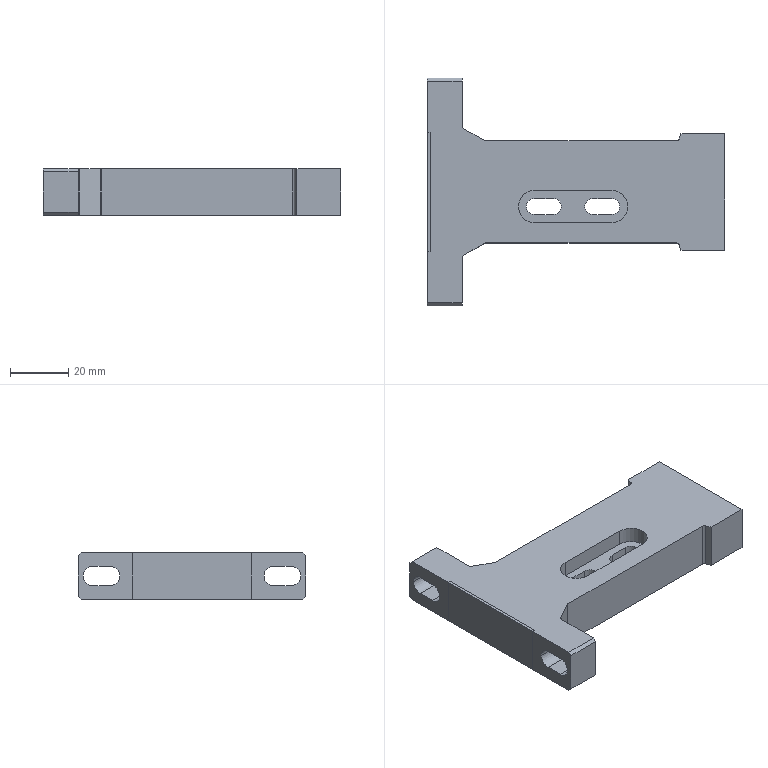NC program | NX | posted with a generic post | part box 102 x 78 x 16 mm
Lines 1 to 22 of 11044:
N10 G17 G21 G94 G90
(FLOOR_WALL , TOOL : D63)
N12 T01 M6
N14 G54
N16 G17 G0 G90 X-88.5 Y41.997 B0. C0. S6500 M3
N18 G43 Z30. H1
N20 Z3.
N22 G94 G1 Z0. F1250.
N24 X-85.5
N26 X85.5
N28 Y12.599
N30 X-85.5
N32 Y-16.8
N34 X85.5
N36 X88.5
N38 Z3.
N40 G0 Z30.
N42 M5